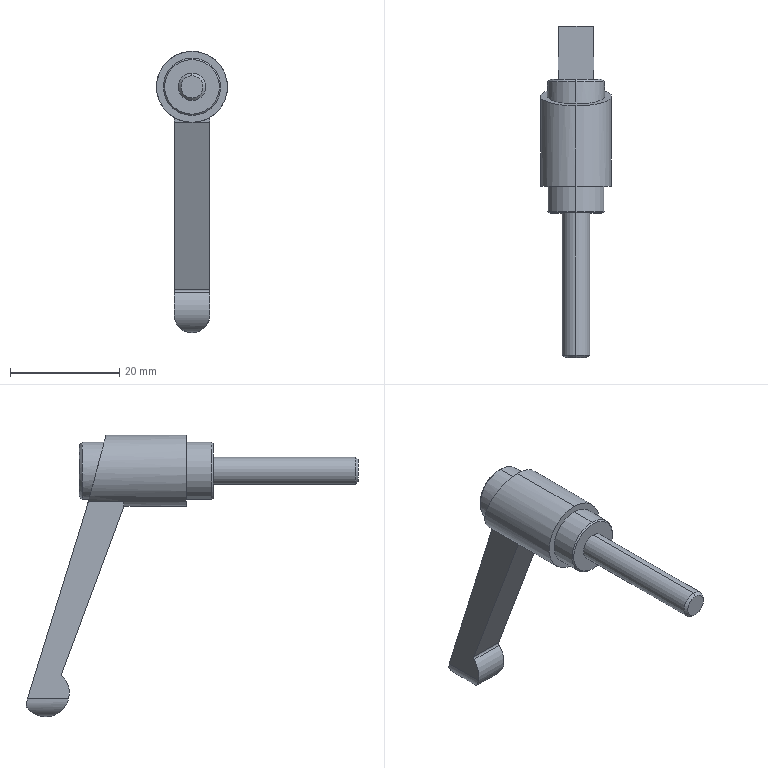Part | NX | features BREP 1 | 1 solid | 31 faces | box 13 x 60.763 x 51.5 mm | volume 4863 mm3 | cylinder 14 | plane 11 | cone 6 | commonest cylinder face diameters 10.5 x4 5 x2 6.5 x2 8.667 x2 13 x2 1 x1
STEP:
#1=CARTESIAN_POINT('',(0.,30.667,-45.));
#2=VERTEX_POINT('',#1);
#3=CARTESIAN_POINT('',(2.806,34.038,-43.389));
#4=VERTEX_POINT('',#3);
#5=CARTESIAN_POINT('',(2.806,34.038,-43.389));
#6=CARTESIAN_POINT('',(2.68,33.863,-43.606));
#7=CARTESIAN_POINT('',(2.372,33.461,-44.024));
#8=CARTESIAN_POINT('',(1.815,32.783,-44.468));
#9=CARTESIAN_POINT('',(1.358,32.244,-44.714));
#10=CARTESIAN_POINT('',(0.9002,31.708,-44.884));
#11=CARTESIAN_POINT('',(0.5923,31.35,-44.948));
#12=CARTESIAN_POINT('',(0.3641,31.087,-44.983));
#13=CARTESIAN_POINT('',(0.1339,30.821,-45.));
#14=CARTESIAN_POINT('',(0.,30.667,-45.));
#15=B_SPLINE_CURVE_WITH_KNOTS('',3,(#5,#6,#7,#8,#9,#10,#11,#12,#13,#14),.UNSPECIFIED.,.F.,.F.,(4,1,1,1,1,1,1,4),(0.,0.25,0.5,0.625,0.75,0.875,0.9375,1.),.UNSPECIFIED.);
#16=EDGE_CURVE('',#2,#4,#15,.F.);
#17=ORIENTED_EDGE('',*,*,#16,.F.);
#18=CARTESIAN_POINT('',(-2.806,34.038,-43.389));
#19=VERTEX_POINT('',#18);
#20=CARTESIAN_POINT('',(0.,30.667,-45.));
#21=CARTESIAN_POINT('',(-0.1339,30.821,-45.));
#22=CARTESIAN_POINT('',(-0.3641,31.087,-44.983));
#23=CARTESIAN_POINT('',(-0.5923,31.35,-44.948));
#24=CARTESIAN_POINT('',(-0.9002,31.708,-44.884));
#25=CARTESIAN_POINT('',(-1.358,32.244,-44.714));
#26=CARTESIAN_POINT('',(-1.815,32.783,-44.468));
#27=CARTESIAN_POINT('',(-2.372,33.461,-44.024));
#28=CARTESIAN_POINT('',(-2.68,33.863,-43.606));
#29=CARTESIAN_POINT('',(-2.806,34.038,-43.389));
#30=B_SPLINE_CURVE_WITH_KNOTS('',3,(#20,#21,#22,#23,#24,#25,#26,#27,#28,#29),.UNSPECIFIED.,.F.,.F.,(4,1,1,1,1,1,1,4),(0.,0.0625,0.125,0.25,0.375,0.5,0.75,1.),.UNSPECIFIED.);
#31=EDGE_CURVE('',#19,#2,#30,.F.);
#32=ORIENTED_EDGE('',*,*,#31,.F.);
#33=CARTESIAN_POINT('',(-2.806,34.038,-43.389));
#34=DIRECTION('',(1.,0.,0.));
#35=VECTOR('',#34,1000.);
#36=LINE('',#33,#35);
#37=EDGE_CURVE('',#19,#4,#36,.T.);
#38=ORIENTED_EDGE('',*,*,#37,.T.);
#39=EDGE_LOOP('',(#17,#32,#38));
#40=FACE_BOUND('',#39,.T.);
#41=CARTESIAN_POINT('',(3.25,30.667,-40.667));
#42=DIRECTION('',(1.,0.,0.));
#43=DIRECTION('',(0.,0.,1.));
#44=AXIS2_PLACEMENT_3D('',#41,#42,#43);
#45=CYLINDRICAL_SURFACE('',#44,4.333);
#46=ADVANCED_FACE('',(#40),#45,.T.);
#47=CARTESIAN_POINT('',(-3.17,34.215,-42.465));
#48=VERTEX_POINT('',#47);
#49=CARTESIAN_POINT('',(-2.806,34.038,-43.389));
#50=CARTESIAN_POINT('',(-2.874,34.132,-43.273));
#51=CARTESIAN_POINT('',(-2.908,34.16,-43.204));
#52=CARTESIAN_POINT('',(-3.07,34.29,-42.852));
#53=CARTESIAN_POINT('',(-3.137,34.261,-42.614));
#54=CARTESIAN_POINT('',(-3.17,34.215,-42.465));
#55=B_SPLINE_CURVE_WITH_KNOTS('',3,(#49,#50,#51,#52,#53,#54),.UNSPECIFIED.,.F.,.F.,(4,1,1,4),(0.,0.25,0.5,1.),.UNSPECIFIED.);
#56=EDGE_CURVE('',#48,#19,#55,.F.);
#57=ORIENTED_EDGE('',*,*,#56,.F.);
#58=CARTESIAN_POINT('',(3.17,34.215,-42.465));
#59=VERTEX_POINT('',#58);
#60=CARTESIAN_POINT('',(-3.17,34.215,-42.465));
#61=DIRECTION('',(1.,0.,0.));
#62=VECTOR('',#61,1000.);
#63=LINE('',#60,#62);
#64=EDGE_CURVE('',#48,#59,#63,.T.);
#65=ORIENTED_EDGE('',*,*,#64,.T.);
#66=CARTESIAN_POINT('',(3.17,34.215,-42.465));
#67=CARTESIAN_POINT('',(3.137,34.261,-42.614));
#68=CARTESIAN_POINT('',(3.04,34.261,-42.914));
#69=CARTESIAN_POINT('',(2.957,34.208,-43.099));
#70=CARTESIAN_POINT('',(2.862,34.115,-43.294));
#71=CARTESIAN_POINT('',(2.806,34.038,-43.389));
#72=B_SPLINE_CURVE_WITH_KNOTS('',3,(#66,#67,#68,#69,#70,#71),.UNSPECIFIED.,.F.,.F.,(4,1,1,4),(0.,0.5,0.75,1.),.UNSPECIFIED.);
#73=EDGE_CURVE('',#4,#59,#72,.F.);
#74=ORIENTED_EDGE('',*,*,#73,.F.);
#75=ORIENTED_EDGE('',*,*,#37,.F.);
#76=EDGE_LOOP('',(#57,#65,#74,#75));
#77=FACE_BOUND('',#76,.T.);
#78=CARTESIAN_POINT('',(3.25,33.26,-42.761));
#79=DIRECTION('',(1.,0.,0.));
#80=DIRECTION('',(0.,0.,1.));
#81=AXIS2_PLACEMENT_3D('',#78,#79,#80);
#82=CYLINDRICAL_SURFACE('',#81,1.);
#83=ADVANCED_FACE('',(#77),#82,.T.);
#84=ORIENTED_EDGE('',*,*,#73,.T.);
#85=CARTESIAN_POINT('',(3.25,33.994,-41.75));
#86=VERTEX_POINT('',#85);
#87=CARTESIAN_POINT('',(3.25,33.994,-41.75));
#88=CARTESIAN_POINT('',(3.25,34.069,-41.991));
#89=CARTESIAN_POINT('',(3.223,34.143,-42.23));
#90=CARTESIAN_POINT('',(3.17,34.215,-42.465));
#91=B_SPLINE_CURVE_WITH_KNOTS('',3,(#87,#88,#89,#90),.UNSPECIFIED.,.F.,.F.,(4,4),(0.,1.),.UNSPECIFIED.);
#92=EDGE_CURVE('',#59,#86,#91,.F.);
#93=ORIENTED_EDGE('',*,*,#92,.T.);
#94=CARTESIAN_POINT('',(3.25,26.471,-41.75));
#95=VERTEX_POINT('',#94);
#96=CARTESIAN_POINT('',(3.25,33.994,-41.75));
#97=DIRECTION('',(0.,-1.,0.));
#98=VECTOR('',#97,1000.);
#99=LINE('',#96,#98);
#100=EDGE_CURVE('',#86,#95,#99,.T.);
#101=ORIENTED_EDGE('',*,*,#100,.T.);
#102=CARTESIAN_POINT('',(3.25,26.471,-41.75));
#103=CARTESIAN_POINT('',(3.25,26.568,-42.126));
#104=CARTESIAN_POINT('',(3.136,26.847,-42.848));
#105=CARTESIAN_POINT('',(2.601,27.583,-43.769));
#106=CARTESIAN_POINT('',(2.022,28.302,-44.324));
#107=CARTESIAN_POINT('',(1.505,28.917,-44.644));
#108=CARTESIAN_POINT('',(1.128,29.36,-44.806));
#109=CARTESIAN_POINT('',(0.7305,29.822,-44.923));
#110=CARTESIAN_POINT('',(0.4776,30.116,-44.97));
#111=CARTESIAN_POINT('',(0.1691,30.471,-45.));
#112=CARTESIAN_POINT('',(0.,30.667,-45.));
#113=B_SPLINE_CURVE_WITH_KNOTS('',3,(#102,#103,#104,#105,#106,#107,#108,#109,#110,#111,#112),.UNSPECIFIED.,.F.,.F.,(4,1,1,1,1,1,1,1,4),(0.,0.25,0.5,0.625,0.75,0.8125,0.875,0.9375,1.),.UNSPECIFIED.);
#114=EDGE_CURVE('',#95,#2,#113,.T.);
#115=ORIENTED_EDGE('',*,*,#114,.T.);
#116=ORIENTED_EDGE('',*,*,#16,.T.);
#117=EDGE_LOOP('',(#84,#93,#101,#115,#116));
#118=FACE_BOUND('',#117,.T.);
#119=CARTESIAN_POINT('',(0.,35.,-41.75));
#120=DIRECTION('',(0.,1.,0.));
#121=DIRECTION('',(0.,0.,-1.));
#122=AXIS2_PLACEMENT_3D('',#119,#120,#121);
#123=CYLINDRICAL_SURFACE('',#122,3.25);
#124=ADVANCED_FACE('',(#118),#123,.T.);
#125=CARTESIAN_POINT('',(-3.25,26.471,-41.75));
#126=VERTEX_POINT('',#125);
#127=CARTESIAN_POINT('',(-3.25,26.471,-41.75));
#128=CARTESIAN_POINT('',(-3.25,26.566,-42.119));
#129=CARTESIAN_POINT('',(-3.142,26.839,-42.834));
#130=CARTESIAN_POINT('',(-2.604,27.58,-43.767));
#131=CARTESIAN_POINT('',(-2.021,28.302,-44.325));
#132=CARTESIAN_POINT('',(-1.504,28.918,-44.645));
#133=CARTESIAN_POINT('',(-1.118,29.371,-44.809));
#134=CARTESIAN_POINT('',(-0.7337,29.818,-44.923));
#135=CARTESIAN_POINT('',(-0.4511,30.146,-44.971));
#136=CARTESIAN_POINT('',(-0.2193,30.413,-45.));
#137=CARTESIAN_POINT('',(0.,30.667,-45.));
#138=B_SPLINE_CURVE_WITH_KNOTS('',3,(#127,#128,#129,#130,#131,#132,#133,#134,#135,#136,#137),.UNSPECIFIED.,.F.,.F.,(4,1,1,1,1,1,1,1,4),(0.,0.25,0.5,0.625,0.75,0.8125,0.875,0.9375,1.),.UNSPECIFIED.);
#139=EDGE_CURVE('',#2,#126,#138,.F.);
#140=ORIENTED_EDGE('',*,*,#139,.F.);
#141=ORIENTED_EDGE('',*,*,#114,.F.);
#142=CARTESIAN_POINT('',(3.25,27.602,-37.604));
#143=VERTEX_POINT('',#142);
#144=CARTESIAN_POINT('',(3.25,30.667,-40.667));
#145=DIRECTION('',(1.,0.,0.));
#146=DIRECTION('',(0.,-0.7073,0.7069));
#147=AXIS2_PLACEMENT_3D('',#144,#145,#146);
#148=CIRCLE('',#147,4.333);
#149=EDGE_CURVE('',#143,#95,#148,.T.);
#150=ORIENTED_EDGE('',*,*,#149,.F.);
#151=CARTESIAN_POINT('',(-3.25,27.602,-37.604));
#152=VERTEX_POINT('',#151);
#153=CARTESIAN_POINT('',(-3.25,27.602,-37.604));
#154=DIRECTION('',(1.,0.,0.));
#155=VECTOR('',#154,1000.);
#156=LINE('',#153,#155);
#157=EDGE_CURVE('',#152,#143,#156,.T.);
#158=ORIENTED_EDGE('',*,*,#157,.F.);
#159=CARTESIAN_POINT('',(-3.25,30.667,-40.667));
#160=DIRECTION('',(-1.,0.,0.));
#161=DIRECTION('',(0.,-0.9682,-0.25));
#162=AXIS2_PLACEMENT_3D('',#159,#160,#161);
#163=CIRCLE('',#162,4.333);
#164=EDGE_CURVE('',#126,#152,#163,.T.);
#165=ORIENTED_EDGE('',*,*,#164,.F.);
#166=EDGE_LOOP('',(#140,#141,#150,#158,#165));
#167=FACE_BOUND('',#166,.T.);
#168=CARTESIAN_POINT('',(3.25,30.667,-40.667));
#169=DIRECTION('',(1.,0.,0.));
#170=DIRECTION('',(0.,0.,1.));
#171=AXIS2_PLACEMENT_3D('',#168,#169,#170);
#172=CYLINDRICAL_SURFACE('',#171,4.333);
#173=ADVANCED_FACE('',(#167),#172,.T.);
#174=ORIENTED_EDGE('',*,*,#164,.T.);
#175=CARTESIAN_POINT('',(-3.25,27.716,-37.076));
#176=VERTEX_POINT('',#175);
#177=CARTESIAN_POINT('',(-3.25,27.248,-37.25));
#178=DIRECTION('',(1.,0.,0.));
#179=DIRECTION('',(0.,0.7073,-0.7069));
#180=AXIS2_PLACEMENT_3D('',#177,#178,#179);
#181=CIRCLE('',#180,0.5);
#182=EDGE_CURVE('',#152,#176,#181,.T.);
#183=ORIENTED_EDGE('',*,*,#182,.T.);
#184=CARTESIAN_POINT('',(-3.25,16.333,-6.5));
#185=VERTEX_POINT('',#184);
#186=CARTESIAN_POINT('',(-3.25,27.716,-37.076));
#187=DIRECTION('',(0.,-0.3489,0.9372));
#188=VECTOR('',#187,1000.);
#189=LINE('',#186,#188);
#190=EDGE_CURVE('',#176,#185,#189,.T.);
#191=ORIENTED_EDGE('',*,*,#190,.T.);
#192=CARTESIAN_POINT('',(-3.25,16.333,-5.629));
#193=VERTEX_POINT('',#192);
#194=CARTESIAN_POINT('',(-3.25,16.333,-6.5));
#195=DIRECTION('',(0.,0.,1.));
#196=VECTOR('',#195,1000.);
#197=LINE('',#194,#196);
#198=EDGE_CURVE('',#185,#193,#197,.T.);
#199=ORIENTED_EDGE('',*,*,#198,.T.);
#200=CARTESIAN_POINT('',(-3.25,22.814,-5.629));
#201=VERTEX_POINT('',#200);
#202=CARTESIAN_POINT('',(-3.25,22.814,-5.629));
#203=DIRECTION('',(0.,-1.,0.));
#204=VECTOR('',#203,1000.);
#205=LINE('',#202,#204);
#206=EDGE_CURVE('',#201,#193,#205,.T.);
#207=ORIENTED_EDGE('',*,*,#206,.F.);
#208=CARTESIAN_POINT('',(-3.25,33.994,-41.75));
#209=VERTEX_POINT('',#208);
#210=CARTESIAN_POINT('',(-3.25,22.814,-5.629));
#211=DIRECTION('',(0.,0.2957,-0.9553));
#212=VECTOR('',#211,1000.);
#213=LINE('',#210,#212);
#214=EDGE_CURVE('',#201,#209,#213,.T.);
#215=ORIENTED_EDGE('',*,*,#214,.T.);
#216=CARTESIAN_POINT('',(-3.25,26.471,-41.75));
#217=DIRECTION('',(0.,1.,0.));
#218=VECTOR('',#217,1000.);
#219=LINE('',#216,#218);
#220=EDGE_CURVE('',#126,#209,#219,.T.);
#221=ORIENTED_EDGE('',*,*,#220,.F.);
#222=EDGE_LOOP('',(#174,#183,#191,#199,#207,#215,#221));
#223=FACE_BOUND('',#222,.T.);
#224=CARTESIAN_POINT('',(-3.25,27.248,-37.25));
#225=DIRECTION('',(1.,0.,0.));
#226=DIRECTION('',(0.,1.,0.));
#227=AXIS2_PLACEMENT_3D('',#224,#225,#226);
#228=PLANE('',#227);
#229=ADVANCED_FACE('',(#223),#228,.F.);
#230=ORIENTED_EDGE('',*,*,#31,.T.);
#231=ORIENTED_EDGE('',*,*,#139,.T.);
#232=ORIENTED_EDGE('',*,*,#220,.T.);
#233=CARTESIAN_POINT('',(-3.17,34.215,-42.465));
#234=CARTESIAN_POINT('',(-3.223,34.143,-42.23));
#235=CARTESIAN_POINT('',(-3.25,34.069,-41.991));
#236=CARTESIAN_POINT('',(-3.25,33.994,-41.75));
#237=B_SPLINE_CURVE_WITH_KNOTS('',3,(#233,#234,#235,#236),.UNSPECIFIED.,.F.,.F.,(4,4),(0.,1.),.UNSPECIFIED.);
#238=EDGE_CURVE('',#209,#48,#237,.F.);
#239=ORIENTED_EDGE('',*,*,#238,.T.);
#240=ORIENTED_EDGE('',*,*,#56,.T.);
#241=EDGE_LOOP('',(#230,#231,#232,#239,#240));
#242=FACE_BOUND('',#241,.T.);
#243=CARTESIAN_POINT('',(0.,35.,-41.75));
#244=DIRECTION('',(0.,1.,0.));
#245=DIRECTION('',(0.,0.,-1.));
#246=AXIS2_PLACEMENT_3D('',#243,#244,#245);
#247=CYLINDRICAL_SURFACE('',#246,3.25);
#248=ADVANCED_FACE('',(#242),#247,.T.);
#249=ORIENTED_EDGE('',*,*,#92,.F.);
#250=ORIENTED_EDGE('',*,*,#64,.F.);
#251=ORIENTED_EDGE('',*,*,#238,.F.);
#252=ORIENTED_EDGE('',*,*,#214,.F.);
#253=CARTESIAN_POINT('',(0.,23.083,-6.5));
#254=VERTEX_POINT('',#253);
#255=CARTESIAN_POINT('',(-3.25,22.814,-5.629));
#256=CARTESIAN_POINT('',(-2.251,22.992,-6.206));
#257=CARTESIAN_POINT('',(-1.127,23.083,-6.5));
#258=CARTESIAN_POINT('',(0.,23.083,-6.5));
#259=B_SPLINE_CURVE_WITH_KNOTS('',3,(#255,#256,#257,#258),.UNSPECIFIED.,.F.,.F.,(4,4),(0.,1.),.UNSPECIFIED.);
#260=EDGE_CURVE('',#254,#201,#259,.F.);
#261=ORIENTED_EDGE('',*,*,#260,.F.);
#262=CARTESIAN_POINT('',(3.25,22.814,-5.629));
#263=VERTEX_POINT('',#262);
#264=CARTESIAN_POINT('',(0.,23.083,-6.5));
#265=CARTESIAN_POINT('',(1.126,23.083,-6.5));
#266=CARTESIAN_POINT('',(2.25,22.992,-6.206));
#267=CARTESIAN_POINT('',(3.25,22.814,-5.629));
#268=B_SPLINE_CURVE_WITH_KNOTS('',3,(#264,#265,#266,#267),.UNSPECIFIED.,.F.,.F.,(4,4),(0.,1.),.UNSPECIFIED.);
#269=EDGE_CURVE('',#263,#254,#268,.F.);
#270=ORIENTED_EDGE('',*,*,#269,.F.);
#271=CARTESIAN_POINT('',(3.25,33.994,-41.75));
#272=DIRECTION('',(0.,-0.2957,0.9553));
#273=VECTOR('',#272,1000.);
#274=LINE('',#271,#273);
#275=EDGE_CURVE('',#86,#263,#274,.T.);
#276=ORIENTED_EDGE('',*,*,#275,.F.);
#277=EDGE_LOOP('',(#249,#250,#251,#252,#261,#270,#276));
#278=FACE_BOUND('',#277,.T.);
#279=CARTESIAN_POINT('',(3.25,34.215,-42.465));
#280=DIRECTION('',(0.,-0.9553,-0.2957));
#281=DIRECTION('',(0.,0.2957,-0.9553));
#282=AXIS2_PLACEMENT_3D('',#279,#280,#281);
#283=PLANE('',#282);
#284=ADVANCED_FACE('',(#278),#283,.F.);
#285=ORIENTED_EDGE('',*,*,#100,.F.);
#286=ORIENTED_EDGE('',*,*,#275,.T.);
#287=CARTESIAN_POINT('',(3.25,16.333,-5.629));
#288=VERTEX_POINT('',#287);
#289=CARTESIAN_POINT('',(3.25,16.333,-5.629));
#290=DIRECTION('',(0.,1.,0.));
#291=VECTOR('',#290,1000.);
#292=LINE('',#289,#291);
#293=EDGE_CURVE('',#288,#263,#292,.T.);
#294=ORIENTED_EDGE('',*,*,#293,.F.);
#295=CARTESIAN_POINT('',(3.25,16.333,-6.5));
#296=VERTEX_POINT('',#295);
#297=CARTESIAN_POINT('',(3.25,16.333,-6.5));
#298=DIRECTION('',(0.,0.,1.));
#299=VECTOR('',#298,1000.);
#300=LINE('',#297,#299);
#301=EDGE_CURVE('',#296,#288,#300,.T.);
#302=ORIENTED_EDGE('',*,*,#301,.F.);
#303=CARTESIAN_POINT('',(3.25,27.716,-37.076));
#304=VERTEX_POINT('',#303);
#305=CARTESIAN_POINT('',(3.25,16.333,-6.5));
#306=DIRECTION('',(0.,0.3489,-0.9372));
#307=VECTOR('',#306,1000.);
#308=LINE('',#305,#307);
#309=EDGE_CURVE('',#296,#304,#308,.T.);
#310=ORIENTED_EDGE('',*,*,#309,.T.);
#311=CARTESIAN_POINT('',(3.25,27.248,-37.25));
#312=DIRECTION('',(-1.,0.,0.));
#313=DIRECTION('',(0.,0.9372,0.3489));
#314=AXIS2_PLACEMENT_3D('',#311,#312,#313);
#315=CIRCLE('',#314,0.5);
#316=EDGE_CURVE('',#304,#143,#315,.T.);
#317=ORIENTED_EDGE('',*,*,#316,.T.);
#318=ORIENTED_EDGE('',*,*,#149,.T.);
#319=EDGE_LOOP('',(#285,#286,#294,#302,#310,#317,#318));
#320=FACE_BOUND('',#319,.T.);
#321=CARTESIAN_POINT('',(3.25,27.248,-37.25));
#322=DIRECTION('',(1.,0.,0.));
#323=DIRECTION('',(0.,1.,0.));
#324=AXIS2_PLACEMENT_3D('',#321,#322,#323);
#325=PLANE('',#324);
#326=ADVANCED_FACE('',(#320),#325,.T.);
#327=ORIENTED_EDGE('',*,*,#157,.T.);
#328=ORIENTED_EDGE('',*,*,#316,.F.);
#329=CARTESIAN_POINT('',(3.25,27.716,-37.076));
#330=DIRECTION('',(-1.,0.,0.));
#331=VECTOR('',#330,1000.);
#332=LINE('',#329,#331);
#333=EDGE_CURVE('',#304,#176,#332,.T.);
#334=ORIENTED_EDGE('',*,*,#333,.T.);
#335=ORIENTED_EDGE('',*,*,#182,.F.);
#336=EDGE_LOOP('',(#327,#328,#334,#335));
#337=FACE_BOUND('',#336,.T.);
#338=CARTESIAN_POINT('',(3.25,27.248,-37.25));
#339=DIRECTION('',(1.,0.,0.));
#340=DIRECTION('',(0.,0.,1.));
#341=AXIS2_PLACEMENT_3D('',#338,#339,#340);
#342=CYLINDRICAL_SURFACE('',#341,0.5);
#343=ADVANCED_FACE('',(#337),#342,.F.);
#344=ORIENTED_EDGE('',*,*,#333,.F.);
#345=ORIENTED_EDGE('',*,*,#309,.F.);
#346=CARTESIAN_POINT('',(0.,16.333,-6.5));
#347=VERTEX_POINT('',#346);
#348=CARTESIAN_POINT('',(0.,16.333,-6.5));
#349=DIRECTION('',(1.,0.,0.));
#350=VECTOR('',#349,1000.);
#351=LINE('',#348,#350);
#352=EDGE_CURVE('',#347,#296,#351,.T.);
#353=ORIENTED_EDGE('',*,*,#352,.F.);
#354=CARTESIAN_POINT('',(-3.25,16.333,-6.5));
#355=DIRECTION('',(1.,0.,0.));
#356=VECTOR('',#355,1000.);
#357=LINE('',#354,#356);
#358=EDGE_CURVE('',#185,#347,#357,.T.);
#359=ORIENTED_EDGE('',*,*,#358,.F.);
#360=ORIENTED_EDGE('',*,*,#190,.F.);
#361=EDGE_LOOP('',(#344,#345,#353,#359,#360));
#362=FACE_BOUND('',#361,.T.);
#363=CARTESIAN_POINT('',(3.25,16.333,-6.5));
#364=DIRECTION('',(0.,0.9372,0.3489));
#365=DIRECTION('',(1.,0.,0.));
#366=AXIS2_PLACEMENT_3D('',#363,#364,#365);
#367=PLANE('',#366);
#368=ADVANCED_FACE('',(#362),#367,.F.);
#369=CARTESIAN_POINT('',(0.,16.333,0.));
#370=DIRECTION('',(0.,1.,0.));
#371=DIRECTION('',(0.,0.,-1.));
#372=AXIS2_PLACEMENT_3D('',#369,#370,#371);
#373=CIRCLE('',#372,6.5);
#374=EDGE_CURVE('',#347,#193,#373,.T.);
#375=ORIENTED_EDGE('',*,*,#374,.T.);
#376=ORIENTED_EDGE('',*,*,#198,.F.);
#377=ORIENTED_EDGE('',*,*,#358,.T.);
#378=EDGE_LOOP('',(#375,#376,#377));
#379=FACE_BOUND('',#378,.T.);
#380=CARTESIAN_POINT('',(3.25,16.333,0.));
#381=DIRECTION('',(0.,1.,0.));
#382=DIRECTION('',(1.,0.,0.));
#383=AXIS2_PLACEMENT_3D('',#380,#381,#382);
#384=PLANE('',#383);
#385=ADVANCED_FACE('',(#379),#384,.F.);
#386=ORIENTED_EDGE('',*,*,#260,.T.);
#387=ORIENTED_EDGE('',*,*,#206,.T.);
#388=ORIENTED_EDGE('',*,*,#374,.F.);
#389=CARTESIAN_POINT('',(0.,4.9,-6.5));
#390=VERTEX_POINT('',#389);
#391=CARTESIAN_POINT('',(0.,4.9,-6.5));
#392=DIRECTION('',(0.,1.,0.));
#393=VECTOR('',#392,1000.);
#394=LINE('',#391,#393);
#395=EDGE_CURVE('',#390,#347,#394,.T.);
#396=ORIENTED_EDGE('',*,*,#395,.F.);
#397=CARTESIAN_POINT('',(0.,4.9,6.5));
#398=VERTEX_POINT('',#397);
#399=CARTESIAN_POINT('',(0.,4.9,0.));
#400=DIRECTION('',(0.,-1.,0.));
#401=DIRECTION('',(0.,0.,1.));
#402=AXIS2_PLACEMENT_3D('',#399,#400,#401);
#403=CIRCLE('',#402,6.5);
#404=EDGE_CURVE('',#398,#390,#403,.T.);
#405=ORIENTED_EDGE('',*,*,#404,.F.);
#406=CARTESIAN_POINT('',(0.,19.6,6.5));
#407=VERTEX_POINT('',#406);
#408=CARTESIAN_POINT('',(0.,4.9,6.5));
#409=DIRECTION('',(0.,1.,0.));
#410=VECTOR('',#409,1000.);
#411=LINE('',#408,#410);
#412=EDGE_CURVE('',#398,#407,#411,.T.);
#413=ORIENTED_EDGE('',*,*,#412,.T.);
#414=CARTESIAN_POINT('',(0.,23.083,-6.5));
#415=CARTESIAN_POINT('',(-0.8361,23.083,-6.5));
#416=CARTESIAN_POINT('',(-2.441,23.003,-6.199));
#417=CARTESIAN_POINT('',(-4.728,22.613,-4.744));
#418=CARTESIAN_POINT('',(-6.224,21.986,-2.403));
#419=CARTESIAN_POINT('',(-6.638,21.342,-0.00000186));
#420=CARTESIAN_POINT('',(-6.224,20.698,2.403));
#421=CARTESIAN_POINT('',(-4.728,20.071,4.744));
#422=CARTESIAN_POINT('',(-2.441,19.681,6.199));
#423=CARTESIAN_POINT('',(-0.8364,19.6,6.5));
#424=CARTESIAN_POINT('',(0.,19.6,6.5));
#425=B_SPLINE_CURVE_WITH_KNOTS('',3,(#414,#415,#416,#417,#418,#419,#420,#421,#422,#423,#424),.UNSPECIFIED.,.F.,.F.,(4,1,1,1,1,1,1,1,4),(0.,0.125,0.25,0.375,0.5,0.625,0.75,0.875,1.),.UNSPECIFIED.);
#426=EDGE_CURVE('',#407,#254,#425,.F.);
#427=ORIENTED_EDGE('',*,*,#426,.T.);
#428=EDGE_LOOP('',(#386,#387,#388,#396,#405,#413,#427));
#429=FACE_BOUND('',#428,.T.);
#430=CARTESIAN_POINT('',(0.,-26.5,0.));
#431=DIRECTION('',(0.,1.,0.));
#432=DIRECTION('',(0.,0.,-1.));
#433=AXIS2_PLACEMENT_3D('',#430,#431,#432);
#434=CYLINDRICAL_SURFACE('',#433,6.5);
#435=ADVANCED_FACE('',(#429),#434,.T.);
#436=CARTESIAN_POINT('',(0.,19.6,6.5));
#437=CARTESIAN_POINT('',(0.8361,19.6,6.5));
#438=CARTESIAN_POINT('',(2.441,19.681,6.199));
#439=CARTESIAN_POINT('',(4.728,20.071,4.744));
#440=CARTESIAN_POINT('',(6.224,20.698,2.403));
#441=CARTESIAN_POINT('',(6.638,21.342,0.00000186));
#442=CARTESIAN_POINT('',(6.224,21.986,-2.403));
#443=CARTESIAN_POINT('',(4.728,22.613,-4.744));
#444=CARTESIAN_POINT('',(2.441,23.003,-6.199));
#445=CARTESIAN_POINT('',(0.8364,23.083,-6.5));
#446=CARTESIAN_POINT('',(0.,23.083,-6.5));
#447=B_SPLINE_CURVE_WITH_KNOTS('',3,(#436,#437,#438,#439,#440,#441,#442,#443,#444,#445,#446),.UNSPECIFIED.,.F.,.F.,(4,1,1,1,1,1,1,1,4),(0.,0.125,0.25,0.375,0.5,0.625,0.75,0.875,1.),.UNSPECIFIED.);
#448=EDGE_CURVE('',#254,#407,#447,.F.);
#449=ORIENTED_EDGE('',*,*,#448,.F.);
#450=ORIENTED_EDGE('',*,*,#426,.F.);
#451=EDGE_LOOP('',(#449,#450));
#452=FACE_BOUND('',#451,.T.);
#453=CARTESIAN_POINT('',(0.,19.935,5.25));
#454=VERTEX_POINT('',#453);
#455=CARTESIAN_POINT('',(0.,22.748,-5.25));
#456=VERTEX_POINT('',#455);
#457=CARTESIAN_POINT('',(0.,22.748,-5.25));
#458=CARTESIAN_POINT('',(0.6753,22.748,-5.25));
#459=CARTESIAN_POINT('',(1.972,22.683,-5.007));
#460=CARTESIAN_POINT('',(3.819,22.368,-3.832));
#461=CARTESIAN_POINT('',(5.027,21.862,-1.941));
#462=CARTESIAN_POINT('',(5.361,21.342,-0.00000147));
#463=CARTESIAN_POINT('',(5.027,20.822,1.941));
#464=CARTESIAN_POINT('',(3.819,20.315,3.832));
#465=CARTESIAN_POINT('',(1.972,20.,5.007));
#466=CARTESIAN_POINT('',(0.6757,19.935,5.25));
#467=CARTESIAN_POINT('',(0.,19.935,5.25));
#468=B_SPLINE_CURVE_WITH_KNOTS('',3,(#457,#458,#459,#460,#461,#462,#463,#464,#465,#466,#467),.UNSPECIFIED.,.F.,.F.,(4,1,1,1,1,1,1,1,4),(0.,0.125,0.25,0.375,0.5,0.625,0.75,0.875,1.),.UNSPECIFIED.);
#469=EDGE_CURVE('',#454,#456,#468,.F.);
#470=ORIENTED_EDGE('',*,*,#469,.F.);
#471=CARTESIAN_POINT('',(0.,19.935,5.25));
#472=CARTESIAN_POINT('',(-0.6753,19.935,5.25));
#473=CARTESIAN_POINT('',(-1.972,20.,5.007));
#474=CARTESIAN_POINT('',(-3.819,20.315,3.832));
#475=CARTESIAN_POINT('',(-5.027,20.822,1.941));
#476=CARTESIAN_POINT('',(-5.361,21.342,0.00000147));
#477=CARTESIAN_POINT('',(-5.027,21.862,-1.941));
#478=CARTESIAN_POINT('',(-3.819,22.368,-3.832));
#479=CARTESIAN_POINT('',(-1.972,22.683,-5.007));
#480=CARTESIAN_POINT('',(-0.6757,22.748,-5.25));
#481=CARTESIAN_POINT('',(0.,22.748,-5.25));
#482=B_SPLINE_CURVE_WITH_KNOTS('',3,(#471,#472,#473,#474,#475,#476,#477,#478,#479,#480,#481),.UNSPECIFIED.,.F.,.F.,(4,1,1,1,1,1,1,1,4),(0.,0.125,0.25,0.375,0.5,0.625,0.75,0.875,1.),.UNSPECIFIED.);
#483=EDGE_CURVE('',#456,#454,#482,.F.);
#484=ORIENTED_EDGE('',*,*,#483,.F.);
#485=EDGE_LOOP('',(#470,#484));
#486=FACE_BOUND('',#485,.T.);
#487=CARTESIAN_POINT('',(13.,19.6,6.5));
#488=DIRECTION('',(0.,0.9659,0.2588));
#489=DIRECTION('',(1.,0.,0.));
#490=AXIS2_PLACEMENT_3D('',#487,#488,#489);
#491=PLANE('',#490);
#492=ADVANCED_FACE('',(#452,#486),#491,.T.);
#493=ORIENTED_EDGE('',*,*,#412,.F.);
#494=CARTESIAN_POINT('',(0.,4.9,0.));
#495=DIRECTION('',(0.,-1.,0.));
#496=DIRECTION('',(0.,0.,-1.));
#497=AXIS2_PLACEMENT_3D('',#494,#495,#496);
#498=CIRCLE('',#497,6.5);
#499=EDGE_CURVE('',#390,#398,#498,.T.);
#500=ORIENTED_EDGE('',*,*,#499,.F.);
#501=ORIENTED_EDGE('',*,*,#395,.T.);
#502=CARTESIAN_POINT('',(0.,16.333,0.));
#503=DIRECTION('',(0.,1.,0.));
#504=DIRECTION('',(0.5,0.,-0.866));
#505=AXIS2_PLACEMENT_3D('',#502,#503,#504);
#506=CIRCLE('',#505,6.5);
#507=EDGE_CURVE('',#288,#347,#506,.T.);
#508=ORIENTED_EDGE('',*,*,#507,.F.);
#509=ORIENTED_EDGE('',*,*,#293,.T.);
#510=ORIENTED_EDGE('',*,*,#269,.T.);
#511=ORIENTED_EDGE('',*,*,#448,.T.);
#512=EDGE_LOOP('',(#493,#500,#501,#508,#509,#510,#511));
#513=FACE_BOUND('',#512,.T.);
#514=CARTESIAN_POINT('',(0.,-26.5,0.));
#515=DIRECTION('',(0.,1.,0.));
#516=DIRECTION('',(0.,0.,-1.));
#517=AXIS2_PLACEMENT_3D('',#514,#515,#516);
#518=CYLINDRICAL_SURFACE('',#517,6.5);
#519=ADVANCED_FACE('',(#513),#518,.T.);
#520=ORIENTED_EDGE('',*,*,#507,.T.);
#521=ORIENTED_EDGE('',*,*,#352,.T.);
#522=ORIENTED_EDGE('',*,*,#301,.T.);
#523=EDGE_LOOP('',(#520,#521,#522));
#524=FACE_BOUND('',#523,.T.);
#525=CARTESIAN_POINT('',(3.25,16.333,0.));
#526=DIRECTION('',(0.,1.,0.));
#527=DIRECTION('',(1.,0.,0.));
#528=AXIS2_PLACEMENT_3D('',#525,#526,#527);
#529=PLANE('',#528);
#530=ADVANCED_FACE('',(#524),#529,.F.);
#531=ORIENTED_EDGE('',*,*,#404,.T.);
#532=ORIENTED_EDGE('',*,*,#499,.T.);
#533=EDGE_LOOP('',(#531,#532));
#534=FACE_BOUND('',#533,.T.);
#535=CARTESIAN_POINT('',(0.,4.9,5.25));
#536=VERTEX_POINT('',#535);
#537=CARTESIAN_POINT('',(0.,4.9,-5.25));
#538=VERTEX_POINT('',#537);
#539=CARTESIAN_POINT('',(0.,4.9,0.));
#540=DIRECTION('',(0.,1.,0.));
#541=DIRECTION('',(0.,0.,1.));
#542=AXIS2_PLACEMENT_3D('',#539,#540,#541);
#543=CIRCLE('',#542,5.25);
#544=EDGE_CURVE('',#536,#538,#543,.T.);
#545=ORIENTED_EDGE('',*,*,#544,.T.);
#546=CARTESIAN_POINT('',(0.,4.9,0.));
#547=DIRECTION('',(0.,1.,0.));
#548=DIRECTION('',(0.,0.,-1.));
#549=AXIS2_PLACEMENT_3D('',#546,#547,#548);
#550=CIRCLE('',#549,5.25);
#551=EDGE_CURVE('',#538,#536,#550,.T.);
#552=ORIENTED_EDGE('',*,*,#551,.T.);
#553=EDGE_LOOP('',(#545,#552));
#554=FACE_BOUND('',#553,.T.);
#555=CARTESIAN_POINT('',(0.,4.9,-6.5));
#556=DIRECTION('',(0.,1.,0.));
#557=DIRECTION('',(1.,0.,0.));
#558=AXIS2_PLACEMENT_3D('',#555,#556,#557);
#559=PLANE('',#558);
#560=ADVANCED_FACE('',(#534,#554),#559,.F.);
#561=CARTESIAN_POINT('',(0.,0.25,-5.25));
#562=VERTEX_POINT('',#561);
#563=CARTESIAN_POINT('',(0.,0.25,-5.25));
#564=DIRECTION('',(0.,1.,0.));
#565=VECTOR('',#564,1000.);
#566=LINE('',#563,#565);
#567=EDGE_CURVE('',#562,#538,#566,.T.);
#568=ORIENTED_EDGE('',*,*,#567,.F.);
#569=CARTESIAN_POINT('',(0.,0.25,5.25));
#570=VERTEX_POINT('',#569);
#571=CARTESIAN_POINT('',(0.,0.25,0.));
#572=DIRECTION('',(0.,-1.,0.));
#573=DIRECTION('',(0.,0.,1.));
#574=AXIS2_PLACEMENT_3D('',#571,#572,#573);
#575=CIRCLE('',#574,5.25);
#576=EDGE_CURVE('',#570,#562,#575,.T.);
#577=ORIENTED_EDGE('',*,*,#576,.F.);
#578=CARTESIAN_POINT('',(0.,0.25,5.25));
#579=DIRECTION('',(0.,1.,0.));
#580=VECTOR('',#579,1000.);
#581=LINE('',#578,#580);
#582=EDGE_CURVE('',#570,#536,#581,.T.);
#583=ORIENTED_EDGE('',*,*,#582,.T.);
#584=ORIENTED_EDGE('',*,*,#551,.F.);
#585=EDGE_LOOP('',(#568,#577,#583,#584));
#586=FACE_BOUND('',#585,.T.);
#587=CARTESIAN_POINT('',(0.,-26.5,0.));
#588=DIRECTION('',(0.,1.,0.));
#589=DIRECTION('',(0.,0.,-1.));
#590=AXIS2_PLACEMENT_3D('',#587,#588,#589);
#591=CYLINDRICAL_SURFACE('',#590,5.25);
#592=ADVANCED_FACE('',(#586),#591,.T.);
#593=ORIENTED_EDGE('',*,*,#582,.F.);
#594=CARTESIAN_POINT('',(0.,0.25,0.));
#595=DIRECTION('',(0.,-1.,0.));
#596=DIRECTION('',(0.,0.,-1.));
#597=AXIS2_PLACEMENT_3D('',#594,#595,#596);
#598=CIRCLE('',#597,5.25);
#599=EDGE_CURVE('',#562,#570,#598,.T.);
#600=ORIENTED_EDGE('',*,*,#599,.F.);
#601=ORIENTED_EDGE('',*,*,#567,.T.);
#602=ORIENTED_EDGE('',*,*,#544,.F.);
#603=EDGE_LOOP('',(#593,#600,#601,#602));
#604=FACE_BOUND('',#603,.T.);
#605=CARTESIAN_POINT('',(0.,-26.5,0.));
#606=DIRECTION('',(0.,1.,0.));
#607=DIRECTION('',(0.,0.,-1.));
#608=AXIS2_PLACEMENT_3D('',#605,#606,#607);
#609=CYLINDRICAL_SURFACE('',#608,5.25);
#610=ADVANCED_FACE('',(#604),#609,.T.);
#611=CARTESIAN_POINT('',(0.,0.,5.));
#612=VERTEX_POINT('',#611);
#613=CARTESIAN_POINT('',(0.,0.,5.));
#614=DIRECTION('',(0.,0.7071,0.7071));
#615=VECTOR('',#614,1000.);
#616=LINE('',#613,#615);
#617=EDGE_CURVE('',#570,#612,#616,.F.);
#618=ORIENTED_EDGE('',*,*,#617,.T.);
#619=CARTESIAN_POINT('',(0.,0.,-5.));
#620=VERTEX_POINT('',#619);
#621=CARTESIAN_POINT('',(0.,0.,0.));
#622=DIRECTION('',(0.,-1.,0.));
#623=DIRECTION('',(0.,0.,-1.));
#624=AXIS2_PLACEMENT_3D('',#621,#622,#623);
#625=CIRCLE('',#624,5.);
#626=EDGE_CURVE('',#620,#612,#625,.T.);
#627=ORIENTED_EDGE('',*,*,#626,.F.);
#628=CARTESIAN_POINT('',(0.,0.,-5.));
#629=DIRECTION('',(0.,0.7071,-0.7071));
#630=VECTOR('',#629,1000.);
#631=LINE('',#628,#630);
#632=EDGE_CURVE('',#562,#620,#631,.F.);
#633=ORIENTED_EDGE('',*,*,#632,.F.);
#634=ORIENTED_EDGE('',*,*,#599,.T.);
#635=EDGE_LOOP('',(#618,#627,#633,#634));
#636=FACE_BOUND('',#635,.T.);
#637=CARTESIAN_POINT('',(0.,0.125,0.));
#638=DIRECTION('',(0.,1.,0.));
#639=DIRECTION('',(0.,0.,1.));
#640=AXIS2_PLACEMENT_3D('',#637,#638,#639);
#641=CONICAL_SURFACE('',#640,5.125,0.7854);
#642=ADVANCED_FACE('',(#636),#641,.T.);
#643=ORIENTED_EDGE('',*,*,#632,.T.);
#644=CARTESIAN_POINT('',(0.,0.,0.));
#645=DIRECTION('',(0.,-1.,0.));
#646=DIRECTION('',(0.,0.,1.));
#647=AXIS2_PLACEMENT_3D('',#644,#645,#646);
#648=CIRCLE('',#647,5.);
#649=EDGE_CURVE('',#612,#620,#648,.T.);
#650=ORIENTED_EDGE('',*,*,#649,.F.);
#651=ORIENTED_EDGE('',*,*,#617,.F.);
#652=ORIENTED_EDGE('',*,*,#576,.T.);
#653=EDGE_LOOP('',(#643,#650,#651,#652));
#654=FACE_BOUND('',#653,.T.);
#655=CARTESIAN_POINT('',(0.,0.125,0.));
#656=DIRECTION('',(0.,1.,0.));
#657=DIRECTION('',(0.,0.,1.));
#658=AXIS2_PLACEMENT_3D('',#655,#656,#657);
#659=CONICAL_SURFACE('',#658,5.125,0.7854);
#660=ADVANCED_FACE('',(#654),#659,.T.);
#661=ORIENTED_EDGE('',*,*,#649,.T.);
#662=ORIENTED_EDGE('',*,*,#626,.T.);
#663=EDGE_LOOP('',(#661,#662));
#664=FACE_BOUND('',#663,.T.);
#665=CARTESIAN_POINT('',(0.,0.,2.5));
#666=VERTEX_POINT('',#665);
#667=CARTESIAN_POINT('',(0.,0.,-2.5));
#668=VERTEX_POINT('',#667);
#669=CARTESIAN_POINT('',(0.,0.,0.));
#670=DIRECTION('',(0.,1.,0.));
#671=DIRECTION('',(0.,0.,1.));
#672=AXIS2_PLACEMENT_3D('',#669,#670,#671);
#673=CIRCLE('',#672,2.5);
#674=EDGE_CURVE('',#666,#668,#673,.T.);
#675=ORIENTED_EDGE('',*,*,#674,.T.);
#676=CARTESIAN_POINT('',(0.,0.,0.));
#677=DIRECTION('',(0.,1.,0.));
#678=DIRECTION('',(0.,0.,-1.));
#679=AXIS2_PLACEMENT_3D('',#676,#677,#678);
#680=CIRCLE('',#679,2.5);
#681=EDGE_CURVE('',#668,#666,#680,.T.);
#682=ORIENTED_EDGE('',*,*,#681,.T.);
#683=EDGE_LOOP('',(#675,#682));
#684=FACE_BOUND('',#683,.T.);
#685=CARTESIAN_POINT('',(0.,0.,-5.));
#686=DIRECTION('',(0.,1.,0.));
#687=DIRECTION('',(1.,0.,0.));
#688=AXIS2_PLACEMENT_3D('',#685,#686,#687);
#689=PLANE('',#688);
#690=ADVANCED_FACE('',(#664,#684),#689,.F.);
#691=CARTESIAN_POINT('',(0.,-26.009,-2.5));
#692=VERTEX_POINT('',#691);
#693=CARTESIAN_POINT('',(0.,-26.009,-2.5));
#694=DIRECTION('',(0.,1.,0.));
#695=VECTOR('',#694,1000.);
#696=LINE('',#693,#695);
#697=EDGE_CURVE('',#692,#668,#696,.T.);
#698=ORIENTED_EDGE('',*,*,#697,.F.);
#699=CARTESIAN_POINT('',(0.,-26.009,2.5));
#700=VERTEX_POINT('',#699);
#701=CARTESIAN_POINT('',(0.,-26.009,0.));
#702=DIRECTION('',(0.,-1.,0.));
#703=DIRECTION('',(0.,0.,1.));
#704=AXIS2_PLACEMENT_3D('',#701,#702,#703);
#705=CIRCLE('',#704,2.5);
#706=EDGE_CURVE('',#700,#692,#705,.T.);
#707=ORIENTED_EDGE('',*,*,#706,.F.);
#708=CARTESIAN_POINT('',(0.,-26.009,2.5));
#709=DIRECTION('',(0.,1.,0.));
#710=VECTOR('',#709,1000.);
#711=LINE('',#708,#710);
#712=EDGE_CURVE('',#700,#666,#711,.T.);
#713=ORIENTED_EDGE('',*,*,#712,.T.);
#714=ORIENTED_EDGE('',*,*,#681,.F.);
#715=EDGE_LOOP('',(#698,#707,#713,#714));
#716=FACE_BOUND('',#715,.T.);
#717=CARTESIAN_POINT('',(0.,-26.5,0.));
#718=DIRECTION('',(0.,1.,0.));
#719=DIRECTION('',(0.,0.,-1.));
#720=AXIS2_PLACEMENT_3D('',#717,#718,#719);
#721=CYLINDRICAL_SURFACE('',#720,2.5);
#722=ADVANCED_FACE('',(#716),#721,.T.);
#723=ORIENTED_EDGE('',*,*,#712,.F.);
#724=CARTESIAN_POINT('',(0.,-26.009,0.));
#725=DIRECTION('',(0.,-1.,0.));
#726=DIRECTION('',(0.,0.,-1.));
#727=AXIS2_PLACEMENT_3D('',#724,#725,#726);
#728=CIRCLE('',#727,2.5);
#729=EDGE_CURVE('',#692,#700,#728,.T.);
#730=ORIENTED_EDGE('',*,*,#729,.F.);
#731=ORIENTED_EDGE('',*,*,#697,.T.);
#732=ORIENTED_EDGE('',*,*,#674,.F.);
#733=EDGE_LOOP('',(#723,#730,#731,#732));
#734=FACE_BOUND('',#733,.T.);
#735=CARTESIAN_POINT('',(0.,-26.5,0.));
#736=DIRECTION('',(0.,1.,0.));
#737=DIRECTION('',(0.,0.,-1.));
#738=AXIS2_PLACEMENT_3D('',#735,#736,#737);
#739=CYLINDRICAL_SURFACE('',#738,2.5);
#740=ADVANCED_FACE('',(#734),#739,.T.);
#741=CARTESIAN_POINT('',(0.,-26.5,2.009));
#742=VERTEX_POINT('',#741);
#743=CARTESIAN_POINT('',(0.,-26.5,2.009));
#744=DIRECTION('',(0.,0.7071,0.7071));
#745=VECTOR('',#744,1000.);
#746=LINE('',#743,#745);
#747=EDGE_CURVE('',#700,#742,#746,.F.);
#748=ORIENTED_EDGE('',*,*,#747,.T.);
#749=CARTESIAN_POINT('',(0.,-26.5,-2.009));
#750=VERTEX_POINT('',#749);
#751=CARTESIAN_POINT('',(0.,-26.5,0.));
#752=DIRECTION('',(0.,-1.,0.));
#753=DIRECTION('',(0.,0.,-1.));
#754=AXIS2_PLACEMENT_3D('',#751,#752,#753);
#755=CIRCLE('',#754,2.009);
#756=EDGE_CURVE('',#750,#742,#755,.T.);
#757=ORIENTED_EDGE('',*,*,#756,.F.);
#758=CARTESIAN_POINT('',(0.,-26.5,-2.009));
#759=DIRECTION('',(0.,0.7071,-0.7071));
#760=VECTOR('',#759,1000.);
#761=LINE('',#758,#760);
#762=EDGE_CURVE('',#692,#750,#761,.F.);
#763=ORIENTED_EDGE('',*,*,#762,.F.);
#764=ORIENTED_EDGE('',*,*,#729,.T.);
#765=EDGE_LOOP('',(#748,#757,#763,#764));
#766=FACE_BOUND('',#765,.T.);
#767=CARTESIAN_POINT('',(0.,-26.255,0.));
#768=DIRECTION('',(0.,1.,0.));
#769=DIRECTION('',(0.,0.,1.));
#770=AXIS2_PLACEMENT_3D('',#767,#768,#769);
#771=CONICAL_SURFACE('',#770,2.255,0.7854);
#772=ADVANCED_FACE('',(#766),#771,.T.);
#773=ORIENTED_EDGE('',*,*,#762,.T.);
#774=CARTESIAN_POINT('',(0.,-26.5,0.));
#775=DIRECTION('',(0.,-1.,0.));
#776=DIRECTION('',(0.,0.,1.));
#777=AXIS2_PLACEMENT_3D('',#774,#775,#776);
#778=CIRCLE('',#777,2.009);
#779=EDGE_CURVE('',#742,#750,#778,.T.);
#780=ORIENTED_EDGE('',*,*,#779,.F.);
#781=ORIENTED_EDGE('',*,*,#747,.F.);
#782=ORIENTED_EDGE('',*,*,#706,.T.);
#783=EDGE_LOOP('',(#773,#780,#781,#782));
#784=FACE_BOUND('',#783,.T.);
#785=CARTESIAN_POINT('',(0.,-26.255,0.));
#786=DIRECTION('',(0.,1.,0.));
#787=DIRECTION('',(0.,0.,1.));
#788=AXIS2_PLACEMENT_3D('',#785,#786,#787);
#789=CONICAL_SURFACE('',#788,2.255,0.7854);
#790=ADVANCED_FACE('',(#784),#789,.T.);
#791=ORIENTED_EDGE('',*,*,#779,.T.);
#792=ORIENTED_EDGE('',*,*,#756,.T.);
#793=EDGE_LOOP('',(#791,#792));
#794=FACE_BOUND('',#793,.T.);
#795=CARTESIAN_POINT('',(0.,-26.5,-2.01));
#796=DIRECTION('',(0.,1.,0.));
#797=DIRECTION('',(1.,0.,0.));
#798=AXIS2_PLACEMENT_3D('',#795,#796,#797);
#799=PLANE('',#798);
#800=ADVANCED_FACE('',(#794),#799,.F.);
#801=CARTESIAN_POINT('',(0.,24.,-5.25));
#802=VERTEX_POINT('',#801);
#803=CARTESIAN_POINT('',(0.,22.748,-5.25));
#804=DIRECTION('',(0.,1.,0.));
#805=VECTOR('',#804,1000.);
#806=LINE('',#803,#805);
#807=EDGE_CURVE('',#802,#456,#806,.F.);
#808=ORIENTED_EDGE('',*,*,#807,.T.);
#809=ORIENTED_EDGE('',*,*,#483,.T.);
#810=CARTESIAN_POINT('',(0.,24.,5.25));
#811=VERTEX_POINT('',#810);
#812=CARTESIAN_POINT('',(0.,19.935,5.25));
#813=DIRECTION('',(0.,1.,0.));
#814=VECTOR('',#813,1000.);
#815=LINE('',#812,#814);
#816=EDGE_CURVE('',#811,#454,#815,.F.);
#817=ORIENTED_EDGE('',*,*,#816,.F.);
#818=CARTESIAN_POINT('',(0.,24.,0.));
#819=DIRECTION('',(0.,1.,0.));
#820=DIRECTION('',(0.,0.,-1.));
#821=AXIS2_PLACEMENT_3D('',#818,#819,#820);
#822=CIRCLE('',#821,5.25);
#823=EDGE_CURVE('',#802,#811,#822,.T.);
#824=ORIENTED_EDGE('',*,*,#823,.F.);
#825=EDGE_LOOP('',(#808,#809,#817,#824));
#826=FACE_BOUND('',#825,.T.);
#827=CARTESIAN_POINT('',(0.,12.25,0.));
#828=DIRECTION('',(0.,1.,0.));
#829=DIRECTION('',(0.,0.,-1.));
#830=AXIS2_PLACEMENT_3D('',#827,#828,#829);
#831=CYLINDRICAL_SURFACE('',#830,5.25);
#832=ADVANCED_FACE('',(#826),#831,.T.);
#833=CARTESIAN_POINT('',(0.,24.5,4.75));
#834=VERTEX_POINT('',#833);
#835=CARTESIAN_POINT('',(0.,24.5,4.75));
#836=DIRECTION('',(0.,-0.7071,0.7071));
#837=VECTOR('',#836,1000.);
#838=LINE('',#835,#837);
#839=EDGE_CURVE('',#811,#834,#838,.F.);
#840=ORIENTED_EDGE('',*,*,#839,.T.);
#841=CARTESIAN_POINT('',(0.,24.5,-4.75));
#842=VERTEX_POINT('',#841);
#843=CARTESIAN_POINT('',(0.,24.5,0.));
#844=DIRECTION('',(0.,1.,0.));
#845=DIRECTION('',(0.,0.,-1.));
#846=AXIS2_PLACEMENT_3D('',#843,#844,#845);
#847=CIRCLE('',#846,4.75);
#848=EDGE_CURVE('',#842,#834,#847,.T.);
#849=ORIENTED_EDGE('',*,*,#848,.F.);
#850=CARTESIAN_POINT('',(0.,24.5,-4.75));
#851=DIRECTION('',(0.,-0.7071,-0.7071));
#852=VECTOR('',#851,1000.);
#853=LINE('',#850,#852);
#854=EDGE_CURVE('',#802,#842,#853,.F.);
#855=ORIENTED_EDGE('',*,*,#854,.F.);
#856=ORIENTED_EDGE('',*,*,#823,.T.);
#857=EDGE_LOOP('',(#840,#849,#855,#856));
#858=FACE_BOUND('',#857,.T.);
#859=CARTESIAN_POINT('',(0.,24.25,0.));
#860=DIRECTION('',(0.,-1.,0.));
#861=DIRECTION('',(0.,0.,-1.));
#862=AXIS2_PLACEMENT_3D('',#859,#860,#861);
#863=CONICAL_SURFACE('',#862,5.,0.7854);
#864=ADVANCED_FACE('',(#858),#863,.T.);
#865=ORIENTED_EDGE('',*,*,#854,.T.);
#866=CARTESIAN_POINT('',(0.,24.5,0.));
#867=DIRECTION('',(0.,1.,0.));
#868=DIRECTION('',(0.,0.,1.));
#869=AXIS2_PLACEMENT_3D('',#866,#867,#868);
#870=CIRCLE('',#869,4.75);
#871=EDGE_CURVE('',#834,#842,#870,.T.);
#872=ORIENTED_EDGE('',*,*,#871,.F.);
#873=ORIENTED_EDGE('',*,*,#839,.F.);
#874=CARTESIAN_POINT('',(0.,24.,0.));
#875=DIRECTION('',(0.,1.,0.));
#876=DIRECTION('',(0.,0.,1.));
#877=AXIS2_PLACEMENT_3D('',#874,#875,#876);
#878=CIRCLE('',#877,5.25);
#879=EDGE_CURVE('',#811,#802,#878,.T.);
#880=ORIENTED_EDGE('',*,*,#879,.T.);
#881=EDGE_LOOP('',(#865,#872,#873,#880));
#882=FACE_BOUND('',#881,.T.);
#883=CARTESIAN_POINT('',(0.,24.25,0.));
#884=DIRECTION('',(0.,-1.,0.));
#885=DIRECTION('',(0.,0.,-1.));
#886=AXIS2_PLACEMENT_3D('',#883,#884,#885);
#887=CONICAL_SURFACE('',#886,5.,0.7854);
#888=ADVANCED_FACE('',(#882),#887,.T.);
#889=ORIENTED_EDGE('',*,*,#816,.T.);
#890=ORIENTED_EDGE('',*,*,#469,.T.);
#891=ORIENTED_EDGE('',*,*,#807,.F.);
#892=ORIENTED_EDGE('',*,*,#879,.F.);
#893=EDGE_LOOP('',(#889,#890,#891,#892));
#894=FACE_BOUND('',#893,.T.);
#895=CARTESIAN_POINT('',(0.,12.25,0.));
#896=DIRECTION('',(0.,1.,0.));
#897=DIRECTION('',(0.,0.,-1.));
#898=AXIS2_PLACEMENT_3D('',#895,#896,#897);
#899=CYLINDRICAL_SURFACE('',#898,5.25);
#900=ADVANCED_FACE('',(#894),#899,.T.);
#901=ORIENTED_EDGE('',*,*,#871,.T.);
#902=ORIENTED_EDGE('',*,*,#848,.T.);
#903=EDGE_LOOP('',(#901,#902));
#904=FACE_BOUND('',#903,.T.);
#905=CARTESIAN_POINT('',(0.,24.5,0.));
#906=DIRECTION('',(0.,-1.,0.));
#907=DIRECTION('',(0.,0.,-1.));
#908=AXIS2_PLACEMENT_3D('',#905,#906,#907);
#909=PLANE('',#908);
#910=ADVANCED_FACE('',(#904),#909,.F.);
#911=CLOSED_SHELL('',(#46,#83,#124,#173,#229,#248,#284,#326,#343,#368,#385,#435,#492,#519,#530,#560,#592,#610,#642,#660,#690,#722,#740,#772,#790,#800,#832,#864,#888,#900,#910));
#912=MANIFOLD_SOLID_BREP('',#911);
#913=(LENGTH_UNIT()NAMED_UNIT(*)SI_UNIT(.MILLI.,.METRE.));
#914=UNCERTAINTY_MEASURE_WITH_UNIT(LENGTH_MEASURE(0.0508),#913,'','');
#915=(NAMED_UNIT(*)PLANE_ANGLE_UNIT()SI_UNIT($,.RADIAN.));
#916=(NAMED_UNIT(*)SI_UNIT($,.STERADIAN.)SOLID_ANGLE_UNIT());
#917=(GEOMETRIC_REPRESENTATION_CONTEXT(3)GLOBAL_UNCERTAINTY_ASSIGNED_CONTEXT((#914))GLOBAL_UNIT_ASSIGNED_CONTEXT((#913,#915,#916))REPRESENTATION_CONTEXT('',''));
#918=ADVANCED_BREP_SHAPE_REPRESENTATION('',(#912),#917);